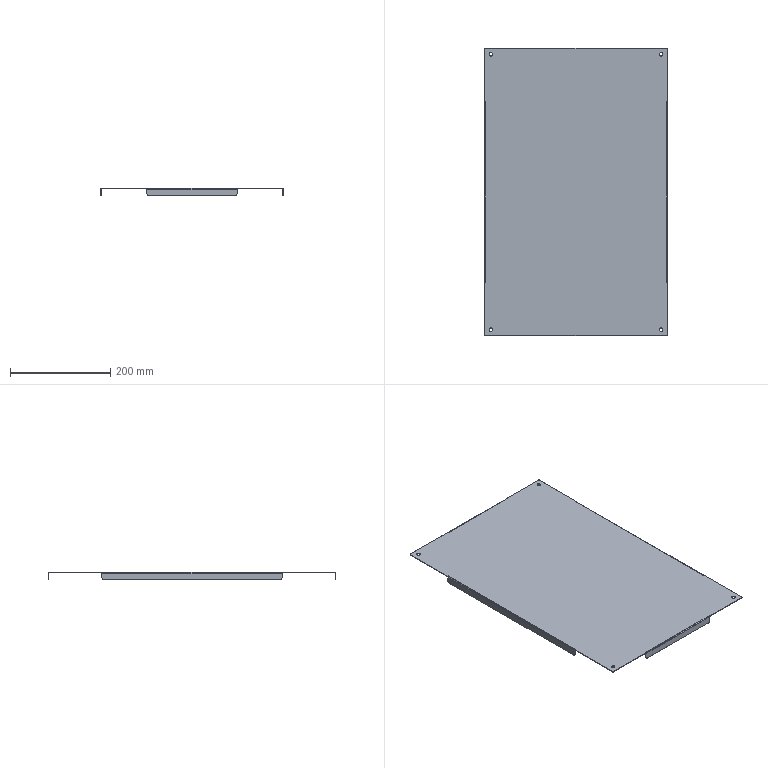Part | SolidWorks | features BaseBody 1 | 1 solid | 90 faces | box 365 x 575 x 15 mm | volume 268880 mm3 | plane 62 | cylinder 28 | commonest cylinder face diameters 7 x8 10 x8 1 x4 3.4 x4 4 x4